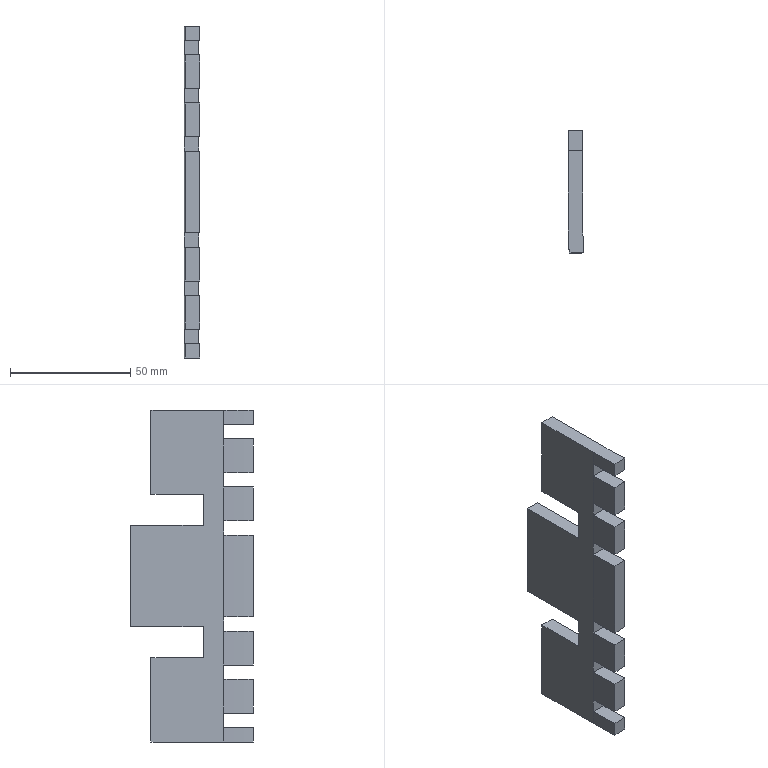Part | SolidWorks | features ICE 2, Extrusion 1 | 1 solid | 52 faces | box 6.316 x 51.1 x 138 mm | volume 31263 mm3 | plane 38 | cylinder 14 | commonest cylinder face diameters 461 x7 473 x7
STEP:
#1=CARTESIAN_POINT('',(-236.5,0.,69.));
#2=VERTEX_POINT('',#1);
#3=CARTESIAN_POINT('',(-236.5,0.,63.));
#4=VERTEX_POINT('',#3);
#5=CARTESIAN_POINT('',(-236.5,0.,69.));
#6=DIRECTION('',(0.,0.,-1.));
#7=VECTOR('',#6,1000.);
#8=LINE('',#5,#7);
#9=EDGE_CURVE('',#2,#4,#8,.T.);
#10=ORIENTED_EDGE('',*,*,#9,.T.);
#11=CARTESIAN_POINT('',(-236.176,-12.377,63.));
#12=VERTEX_POINT('',#11);
#13=CARTESIAN_POINT('',(0.,0.,63.));
#14=DIRECTION('',(0.,0.,1.));
#15=DIRECTION('',(1.,0.,0.));
#16=AXIS2_PLACEMENT_3D('',#13,#14,#15);
#17=CIRCLE('',#16,236.5);
#18=EDGE_CURVE('',#4,#12,#17,.T.);
#19=ORIENTED_EDGE('',*,*,#18,.T.);
#20=CARTESIAN_POINT('',(-236.176,-12.377,69.));
#21=VERTEX_POINT('',#20);
#22=CARTESIAN_POINT('',(-236.176,-12.377,69.));
#23=DIRECTION('',(0.,0.,-1.));
#24=VECTOR('',#23,1000.);
#25=LINE('',#22,#24);
#26=EDGE_CURVE('',#21,#12,#25,.T.);
#27=ORIENTED_EDGE('',*,*,#26,.F.);
#28=CARTESIAN_POINT('',(0.,0.,69.));
#29=DIRECTION('',(0.,0.,1.));
#30=DIRECTION('',(1.,0.,0.));
#31=AXIS2_PLACEMENT_3D('',#28,#29,#30);
#32=CIRCLE('',#31,236.5);
#33=EDGE_CURVE('',#2,#21,#32,.T.);
#34=ORIENTED_EDGE('',*,*,#33,.F.);
#35=EDGE_LOOP('',(#10,#19,#27,#34));
#36=FACE_OUTER_BOUND('',#35,.T.);
#37=CARTESIAN_POINT('',(0.,0.,69.));
#38=DIRECTION('',(0.,0.,-1.));
#39=DIRECTION('',(-1.,0.,0.));
#40=AXIS2_PLACEMENT_3D('',#37,#38,#39);
#41=CYLINDRICAL_SURFACE('',#40,236.5);
#42=ADVANCED_FACE('',(#36),#41,.T.);
#43=CARTESIAN_POINT('',(-236.176,-12.377,57.));
#44=VERTEX_POINT('',#43);
#45=CARTESIAN_POINT('',(-236.176,-12.377,43.));
#46=VERTEX_POINT('',#45);
#47=CARTESIAN_POINT('',(-236.176,-12.377,69.));
#48=DIRECTION('',(0.,0.,-1.));
#49=VECTOR('',#48,1000.);
#50=LINE('',#47,#49);
#51=EDGE_CURVE('',#44,#46,#50,.T.);
#52=ORIENTED_EDGE('',*,*,#51,.F.);
#53=CARTESIAN_POINT('',(-236.5,0.,57.));
#54=VERTEX_POINT('',#53);
#55=CARTESIAN_POINT('',(0.,0.,57.));
#56=DIRECTION('',(0.,0.,-1.));
#57=DIRECTION('',(-1.,0.,0.));
#58=AXIS2_PLACEMENT_3D('',#55,#56,#57);
#59=CIRCLE('',#58,236.5);
#60=EDGE_CURVE('',#44,#54,#59,.T.);
#61=ORIENTED_EDGE('',*,*,#60,.T.);
#62=CARTESIAN_POINT('',(-236.5,0.,43.));
#63=VERTEX_POINT('',#62);
#64=CARTESIAN_POINT('',(-236.5,0.,69.));
#65=DIRECTION('',(0.,0.,-1.));
#66=VECTOR('',#65,1000.);
#67=LINE('',#64,#66);
#68=EDGE_CURVE('',#54,#63,#67,.T.);
#69=ORIENTED_EDGE('',*,*,#68,.T.);
#70=CARTESIAN_POINT('',(0.,0.,43.));
#71=DIRECTION('',(0.,0.,1.));
#72=DIRECTION('',(1.,0.,0.));
#73=AXIS2_PLACEMENT_3D('',#70,#71,#72);
#74=CIRCLE('',#73,236.5);
#75=EDGE_CURVE('',#63,#46,#74,.T.);
#76=ORIENTED_EDGE('',*,*,#75,.T.);
#77=EDGE_LOOP('',(#52,#61,#69,#76));
#78=FACE_OUTER_BOUND('',#77,.T.);
#79=CARTESIAN_POINT('',(0.,0.,69.));
#80=DIRECTION('',(0.,0.,-1.));
#81=DIRECTION('',(-1.,0.,0.));
#82=AXIS2_PLACEMENT_3D('',#79,#80,#81);
#83=CYLINDRICAL_SURFACE('',#82,236.5);
#84=ADVANCED_FACE('',(#78),#83,.T.);
#85=CARTESIAN_POINT('',(-236.176,-12.377,37.));
#86=VERTEX_POINT('',#85);
#87=CARTESIAN_POINT('',(-236.176,-12.377,23.));
#88=VERTEX_POINT('',#87);
#89=CARTESIAN_POINT('',(-236.176,-12.377,69.));
#90=DIRECTION('',(0.,0.,-1.));
#91=VECTOR('',#90,1000.);
#92=LINE('',#89,#91);
#93=EDGE_CURVE('',#86,#88,#92,.T.);
#94=ORIENTED_EDGE('',*,*,#93,.F.);
#95=CARTESIAN_POINT('',(-236.5,0.,37.));
#96=VERTEX_POINT('',#95);
#97=CARTESIAN_POINT('',(0.,0.,37.));
#98=DIRECTION('',(0.,0.,-1.));
#99=DIRECTION('',(-1.,0.,0.));
#100=AXIS2_PLACEMENT_3D('',#97,#98,#99);
#101=CIRCLE('',#100,236.5);
#102=EDGE_CURVE('',#86,#96,#101,.T.);
#103=ORIENTED_EDGE('',*,*,#102,.T.);
#104=CARTESIAN_POINT('',(-236.5,0.,23.));
#105=VERTEX_POINT('',#104);
#106=CARTESIAN_POINT('',(-236.5,0.,69.));
#107=DIRECTION('',(0.,0.,-1.));
#108=VECTOR('',#107,1000.);
#109=LINE('',#106,#108);
#110=EDGE_CURVE('',#96,#105,#109,.T.);
#111=ORIENTED_EDGE('',*,*,#110,.T.);
#112=CARTESIAN_POINT('',(0.,0.,23.));
#113=DIRECTION('',(0.,0.,1.));
#114=DIRECTION('',(0.,-1.,0.));
#115=AXIS2_PLACEMENT_3D('',#112,#113,#114);
#116=CIRCLE('',#115,236.5);
#117=EDGE_CURVE('',#105,#88,#116,.T.);
#118=ORIENTED_EDGE('',*,*,#117,.T.);
#119=EDGE_LOOP('',(#94,#103,#111,#118));
#120=FACE_OUTER_BOUND('',#119,.T.);
#121=CARTESIAN_POINT('',(0.,0.,69.));
#122=DIRECTION('',(0.,0.,-1.));
#123=DIRECTION('',(-1.,0.,0.));
#124=AXIS2_PLACEMENT_3D('',#121,#122,#123);
#125=CYLINDRICAL_SURFACE('',#124,236.5);
#126=ADVANCED_FACE('',(#120),#125,.T.);
#127=CARTESIAN_POINT('',(-236.176,-12.377,17.));
#128=VERTEX_POINT('',#127);
#129=CARTESIAN_POINT('',(-236.176,-12.377,-17.));
#130=VERTEX_POINT('',#129);
#131=CARTESIAN_POINT('',(-236.176,-12.377,69.));
#132=DIRECTION('',(0.,0.,-1.));
#133=VECTOR('',#132,1000.);
#134=LINE('',#131,#133);
#135=EDGE_CURVE('',#128,#130,#134,.T.);
#136=ORIENTED_EDGE('',*,*,#135,.F.);
#137=CARTESIAN_POINT('',(-236.5,0.,17.));
#138=VERTEX_POINT('',#137);
#139=CARTESIAN_POINT('',(0.,0.,17.));
#140=DIRECTION('',(0.,0.,-1.));
#141=DIRECTION('',(0.,1.,0.));
#142=AXIS2_PLACEMENT_3D('',#139,#140,#141);
#143=CIRCLE('',#142,236.5);
#144=EDGE_CURVE('',#128,#138,#143,.T.);
#145=ORIENTED_EDGE('',*,*,#144,.T.);
#146=CARTESIAN_POINT('',(-236.5,0.,-17.));
#147=VERTEX_POINT('',#146);
#148=CARTESIAN_POINT('',(-236.5,0.,69.));
#149=DIRECTION('',(0.,0.,-1.));
#150=VECTOR('',#149,1000.);
#151=LINE('',#148,#150);
#152=EDGE_CURVE('',#138,#147,#151,.T.);
#153=ORIENTED_EDGE('',*,*,#152,.T.);
#154=CARTESIAN_POINT('',(0.,0.,-17.));
#155=DIRECTION('',(0.,0.,1.));
#156=DIRECTION('',(1.,0.,0.));
#157=AXIS2_PLACEMENT_3D('',#154,#155,#156);
#158=CIRCLE('',#157,236.5);
#159=EDGE_CURVE('',#147,#130,#158,.T.);
#160=ORIENTED_EDGE('',*,*,#159,.T.);
#161=EDGE_LOOP('',(#136,#145,#153,#160));
#162=FACE_OUTER_BOUND('',#161,.T.);
#163=CARTESIAN_POINT('',(0.,0.,69.));
#164=DIRECTION('',(0.,0.,-1.));
#165=DIRECTION('',(-1.,0.,0.));
#166=AXIS2_PLACEMENT_3D('',#163,#164,#165);
#167=CYLINDRICAL_SURFACE('',#166,236.5);
#168=ADVANCED_FACE('',(#162),#167,.T.);
#169=CARTESIAN_POINT('',(-236.176,-12.377,-23.));
#170=VERTEX_POINT('',#169);
#171=CARTESIAN_POINT('',(-236.176,-12.377,-37.));
#172=VERTEX_POINT('',#171);
#173=CARTESIAN_POINT('',(-236.176,-12.377,69.));
#174=DIRECTION('',(0.,0.,-1.));
#175=VECTOR('',#174,1000.);
#176=LINE('',#173,#175);
#177=EDGE_CURVE('',#170,#172,#176,.T.);
#178=ORIENTED_EDGE('',*,*,#177,.F.);
#179=CARTESIAN_POINT('',(-236.5,0.,-23.));
#180=VERTEX_POINT('',#179);
#181=CARTESIAN_POINT('',(0.,0.,-23.));
#182=DIRECTION('',(0.,0.,-1.));
#183=DIRECTION('',(0.,1.,0.));
#184=AXIS2_PLACEMENT_3D('',#181,#182,#183);
#185=CIRCLE('',#184,236.5);
#186=EDGE_CURVE('',#170,#180,#185,.T.);
#187=ORIENTED_EDGE('',*,*,#186,.T.);
#188=CARTESIAN_POINT('',(-236.5,0.,-37.));
#189=VERTEX_POINT('',#188);
#190=CARTESIAN_POINT('',(-236.5,0.,69.));
#191=DIRECTION('',(0.,0.,-1.));
#192=VECTOR('',#191,1000.);
#193=LINE('',#190,#192);
#194=EDGE_CURVE('',#180,#189,#193,.T.);
#195=ORIENTED_EDGE('',*,*,#194,.T.);
#196=CARTESIAN_POINT('',(0.,0.,-37.));
#197=DIRECTION('',(0.,0.,1.));
#198=DIRECTION('',(0.,-1.,0.));
#199=AXIS2_PLACEMENT_3D('',#196,#197,#198);
#200=CIRCLE('',#199,236.5);
#201=EDGE_CURVE('',#189,#172,#200,.T.);
#202=ORIENTED_EDGE('',*,*,#201,.T.);
#203=EDGE_LOOP('',(#178,#187,#195,#202));
#204=FACE_OUTER_BOUND('',#203,.T.);
#205=CARTESIAN_POINT('',(0.,0.,69.));
#206=DIRECTION('',(0.,0.,-1.));
#207=DIRECTION('',(-1.,0.,0.));
#208=AXIS2_PLACEMENT_3D('',#205,#206,#207);
#209=CYLINDRICAL_SURFACE('',#208,236.5);
#210=ADVANCED_FACE('',(#204),#209,.T.);
#211=CARTESIAN_POINT('',(-236.176,-12.377,-43.));
#212=VERTEX_POINT('',#211);
#213=CARTESIAN_POINT('',(-236.176,-12.377,-57.));
#214=VERTEX_POINT('',#213);
#215=CARTESIAN_POINT('',(-236.176,-12.377,69.));
#216=DIRECTION('',(0.,0.,-1.));
#217=VECTOR('',#216,1000.);
#218=LINE('',#215,#217);
#219=EDGE_CURVE('',#212,#214,#218,.T.);
#220=ORIENTED_EDGE('',*,*,#219,.F.);
#221=CARTESIAN_POINT('',(-236.5,0.,-43.));
#222=VERTEX_POINT('',#221);
#223=CARTESIAN_POINT('',(0.,0.,-43.));
#224=DIRECTION('',(0.,0.,-1.));
#225=DIRECTION('',(0.,1.,0.));
#226=AXIS2_PLACEMENT_3D('',#223,#224,#225);
#227=CIRCLE('',#226,236.5);
#228=EDGE_CURVE('',#212,#222,#227,.T.);
#229=ORIENTED_EDGE('',*,*,#228,.T.);
#230=CARTESIAN_POINT('',(-236.5,0.,-57.));
#231=VERTEX_POINT('',#230);
#232=CARTESIAN_POINT('',(-236.5,0.,69.));
#233=DIRECTION('',(0.,0.,-1.));
#234=VECTOR('',#233,1000.);
#235=LINE('',#232,#234);
#236=EDGE_CURVE('',#222,#231,#235,.T.);
#237=ORIENTED_EDGE('',*,*,#236,.T.);
#238=CARTESIAN_POINT('',(0.,0.,-57.));
#239=DIRECTION('',(0.,0.,1.));
#240=DIRECTION('',(0.,-1.,0.));
#241=AXIS2_PLACEMENT_3D('',#238,#239,#240);
#242=CIRCLE('',#241,236.5);
#243=EDGE_CURVE('',#231,#214,#242,.T.);
#244=ORIENTED_EDGE('',*,*,#243,.T.);
#245=EDGE_LOOP('',(#220,#229,#237,#244));
#246=FACE_OUTER_BOUND('',#245,.T.);
#247=CARTESIAN_POINT('',(0.,0.,69.));
#248=DIRECTION('',(0.,0.,-1.));
#249=DIRECTION('',(-1.,0.,0.));
#250=AXIS2_PLACEMENT_3D('',#247,#248,#249);
#251=CYLINDRICAL_SURFACE('',#250,236.5);
#252=ADVANCED_FACE('',(#246),#251,.T.);
#253=ORIENTED_EDGE('',*,*,#26,.T.);
#254=CARTESIAN_POINT('',(-230.184,-12.063,63.));
#255=VERTEX_POINT('',#254);
#256=CARTESIAN_POINT('',(-236.176,-12.377,63.));
#257=DIRECTION('',(0.9986,0.05234,0.));
#258=VECTOR('',#257,1000.);
#259=LINE('',#256,#258);
#260=EDGE_CURVE('',#12,#255,#259,.T.);
#261=ORIENTED_EDGE('',*,*,#260,.T.);
#262=CARTESIAN_POINT('',(-230.184,-12.063,69.));
#263=VERTEX_POINT('',#262);
#264=CARTESIAN_POINT('',(-230.184,-12.063,69.));
#265=DIRECTION('',(0.,0.,-1.));
#266=VECTOR('',#265,1000.);
#267=LINE('',#264,#266);
#268=EDGE_CURVE('',#263,#255,#267,.T.);
#269=ORIENTED_EDGE('',*,*,#268,.F.);
#270=CARTESIAN_POINT('',(-236.176,-12.377,69.));
#271=DIRECTION('',(0.9986,0.05234,0.));
#272=VECTOR('',#271,1000.);
#273=LINE('',#270,#272);
#274=EDGE_CURVE('',#21,#263,#273,.T.);
#275=ORIENTED_EDGE('',*,*,#274,.F.);
#276=EDGE_LOOP('',(#253,#261,#269,#275));
#277=FACE_OUTER_BOUND('',#276,.T.);
#278=CARTESIAN_POINT('',(-236.176,-12.377,69.));
#279=DIRECTION('',(-0.05234,0.9986,0.));
#280=DIRECTION('',(-0.9986,-0.05234,0.));
#281=AXIS2_PLACEMENT_3D('',#278,#279,#280);
#282=PLANE('',#281);
#283=ADVANCED_FACE('',(#277),#282,.F.);
#284=CARTESIAN_POINT('',(-230.184,-12.063,57.));
#285=VERTEX_POINT('',#284);
#286=CARTESIAN_POINT('',(-230.184,-12.063,43.));
#287=VERTEX_POINT('',#286);
#288=CARTESIAN_POINT('',(-230.184,-12.063,69.));
#289=DIRECTION('',(0.,0.,-1.));
#290=VECTOR('',#289,1000.);
#291=LINE('',#288,#290);
#292=EDGE_CURVE('',#285,#287,#291,.T.);
#293=ORIENTED_EDGE('',*,*,#292,.F.);
#294=CARTESIAN_POINT('',(-236.176,-12.377,57.));
#295=DIRECTION('',(-0.9986,-0.05234,0.));
#296=VECTOR('',#295,1000.);
#297=LINE('',#294,#296);
#298=EDGE_CURVE('',#285,#44,#297,.T.);
#299=ORIENTED_EDGE('',*,*,#298,.T.);
#300=ORIENTED_EDGE('',*,*,#51,.T.);
#301=CARTESIAN_POINT('',(-236.176,-12.377,43.));
#302=DIRECTION('',(0.9986,0.05234,0.));
#303=VECTOR('',#302,1000.);
#304=LINE('',#301,#303);
#305=EDGE_CURVE('',#46,#287,#304,.T.);
#306=ORIENTED_EDGE('',*,*,#305,.T.);
#307=EDGE_LOOP('',(#293,#299,#300,#306));
#308=FACE_OUTER_BOUND('',#307,.T.);
#309=CARTESIAN_POINT('',(-236.176,-12.377,69.));
#310=DIRECTION('',(-0.05234,0.9986,0.));
#311=DIRECTION('',(-0.9986,-0.05234,0.));
#312=AXIS2_PLACEMENT_3D('',#309,#310,#311);
#313=PLANE('',#312);
#314=ADVANCED_FACE('',(#308),#313,.F.);
#315=CARTESIAN_POINT('',(-230.184,-12.063,37.));
#316=VERTEX_POINT('',#315);
#317=CARTESIAN_POINT('',(-230.184,-12.063,23.));
#318=VERTEX_POINT('',#317);
#319=CARTESIAN_POINT('',(-230.184,-12.063,69.));
#320=DIRECTION('',(0.,0.,-1.));
#321=VECTOR('',#320,1000.);
#322=LINE('',#319,#321);
#323=EDGE_CURVE('',#316,#318,#322,.T.);
#324=ORIENTED_EDGE('',*,*,#323,.F.);
#325=CARTESIAN_POINT('',(-236.176,-12.377,37.));
#326=DIRECTION('',(-0.9986,-0.05234,0.));
#327=VECTOR('',#326,1000.);
#328=LINE('',#325,#327);
#329=EDGE_CURVE('',#316,#86,#328,.T.);
#330=ORIENTED_EDGE('',*,*,#329,.T.);
#331=ORIENTED_EDGE('',*,*,#93,.T.);
#332=CARTESIAN_POINT('',(-236.176,-12.377,23.));
#333=DIRECTION('',(0.9986,0.05234,0.));
#334=VECTOR('',#333,1000.);
#335=LINE('',#332,#334);
#336=EDGE_CURVE('',#88,#318,#335,.T.);
#337=ORIENTED_EDGE('',*,*,#336,.T.);
#338=EDGE_LOOP('',(#324,#330,#331,#337));
#339=FACE_OUTER_BOUND('',#338,.T.);
#340=CARTESIAN_POINT('',(-236.176,-12.377,69.));
#341=DIRECTION('',(-0.05234,0.9986,0.));
#342=DIRECTION('',(-0.9986,-0.05234,0.));
#343=AXIS2_PLACEMENT_3D('',#340,#341,#342);
#344=PLANE('',#343);
#345=ADVANCED_FACE('',(#339),#344,.F.);
#346=CARTESIAN_POINT('',(-230.184,-12.063,17.));
#347=VERTEX_POINT('',#346);
#348=CARTESIAN_POINT('',(-230.184,-12.063,-17.));
#349=VERTEX_POINT('',#348);
#350=CARTESIAN_POINT('',(-230.184,-12.063,69.));
#351=DIRECTION('',(0.,0.,-1.));
#352=VECTOR('',#351,1000.);
#353=LINE('',#350,#352);
#354=EDGE_CURVE('',#347,#349,#353,.T.);
#355=ORIENTED_EDGE('',*,*,#354,.F.);
#356=CARTESIAN_POINT('',(-236.176,-12.377,17.));
#357=DIRECTION('',(-0.9986,-0.05234,0.));
#358=VECTOR('',#357,1000.);
#359=LINE('',#356,#358);
#360=EDGE_CURVE('',#347,#128,#359,.T.);
#361=ORIENTED_EDGE('',*,*,#360,.T.);
#362=ORIENTED_EDGE('',*,*,#135,.T.);
#363=CARTESIAN_POINT('',(-236.176,-12.377,-17.));
#364=DIRECTION('',(0.9986,0.05234,0.));
#365=VECTOR('',#364,1000.);
#366=LINE('',#363,#365);
#367=EDGE_CURVE('',#130,#349,#366,.T.);
#368=ORIENTED_EDGE('',*,*,#367,.T.);
#369=EDGE_LOOP('',(#355,#361,#362,#368));
#370=FACE_OUTER_BOUND('',#369,.T.);
#371=CARTESIAN_POINT('',(-236.176,-12.377,69.));
#372=DIRECTION('',(-0.05234,0.9986,0.));
#373=DIRECTION('',(-0.9986,-0.05234,0.));
#374=AXIS2_PLACEMENT_3D('',#371,#372,#373);
#375=PLANE('',#374);
#376=ADVANCED_FACE('',(#370),#375,.F.);
#377=CARTESIAN_POINT('',(-230.184,-12.063,-23.));
#378=VERTEX_POINT('',#377);
#379=CARTESIAN_POINT('',(-230.184,-12.063,-37.));
#380=VERTEX_POINT('',#379);
#381=CARTESIAN_POINT('',(-230.184,-12.063,69.));
#382=DIRECTION('',(0.,0.,-1.));
#383=VECTOR('',#382,1000.);
#384=LINE('',#381,#383);
#385=EDGE_CURVE('',#378,#380,#384,.T.);
#386=ORIENTED_EDGE('',*,*,#385,.F.);
#387=CARTESIAN_POINT('',(-236.176,-12.377,-23.));
#388=DIRECTION('',(-0.9986,-0.05234,0.));
#389=VECTOR('',#388,1000.);
#390=LINE('',#387,#389);
#391=EDGE_CURVE('',#378,#170,#390,.T.);
#392=ORIENTED_EDGE('',*,*,#391,.T.);
#393=ORIENTED_EDGE('',*,*,#177,.T.);
#394=CARTESIAN_POINT('',(-236.176,-12.377,-37.));
#395=DIRECTION('',(0.9986,0.05234,0.));
#396=VECTOR('',#395,1000.);
#397=LINE('',#394,#396);
#398=EDGE_CURVE('',#172,#380,#397,.T.);
#399=ORIENTED_EDGE('',*,*,#398,.T.);
#400=EDGE_LOOP('',(#386,#392,#393,#399));
#401=FACE_OUTER_BOUND('',#400,.T.);
#402=CARTESIAN_POINT('',(-236.176,-12.377,69.));
#403=DIRECTION('',(-0.05234,0.9986,0.));
#404=DIRECTION('',(-0.9986,-0.05234,0.));
#405=AXIS2_PLACEMENT_3D('',#402,#403,#404);
#406=PLANE('',#405);
#407=ADVANCED_FACE('',(#401),#406,.F.);
#408=CARTESIAN_POINT('',(-230.184,-12.063,-43.));
#409=VERTEX_POINT('',#408);
#410=CARTESIAN_POINT('',(-230.184,-12.063,-57.));
#411=VERTEX_POINT('',#410);
#412=CARTESIAN_POINT('',(-230.184,-12.063,69.));
#413=DIRECTION('',(0.,0.,-1.));
#414=VECTOR('',#413,1000.);
#415=LINE('',#412,#414);
#416=EDGE_CURVE('',#409,#411,#415,.T.);
#417=ORIENTED_EDGE('',*,*,#416,.F.);
#418=CARTESIAN_POINT('',(-236.176,-12.377,-43.));
#419=DIRECTION('',(-0.9986,-0.05234,0.));
#420=VECTOR('',#419,1000.);
#421=LINE('',#418,#420);
#422=EDGE_CURVE('',#409,#212,#421,.T.);
#423=ORIENTED_EDGE('',*,*,#422,.T.);
#424=ORIENTED_EDGE('',*,*,#219,.T.);
#425=CARTESIAN_POINT('',(-236.176,-12.377,-57.));
#426=DIRECTION('',(0.9986,0.05234,0.));
#427=VECTOR('',#426,1000.);
#428=LINE('',#425,#427);
#429=EDGE_CURVE('',#214,#411,#428,.T.);
#430=ORIENTED_EDGE('',*,*,#429,.T.);
#431=EDGE_LOOP('',(#417,#423,#424,#430));
#432=FACE_OUTER_BOUND('',#431,.T.);
#433=CARTESIAN_POINT('',(-236.176,-12.377,69.));
#434=DIRECTION('',(-0.05234,0.9986,0.));
#435=DIRECTION('',(-0.9986,-0.05234,0.));
#436=AXIS2_PLACEMENT_3D('',#433,#434,#435);
#437=PLANE('',#436);
#438=ADVANCED_FACE('',(#432),#437,.F.);
#439=ORIENTED_EDGE('',*,*,#268,.T.);
#440=CARTESIAN_POINT('',(-230.5,0.,63.));
#441=VERTEX_POINT('',#440);
#442=CARTESIAN_POINT('',(0.,0.,63.));
#443=DIRECTION('',(0.,0.,-1.));
#444=DIRECTION('',(1.,0.,0.));
#445=AXIS2_PLACEMENT_3D('',#442,#443,#444);
#446=CIRCLE('',#445,230.5);
#447=EDGE_CURVE('',#255,#441,#446,.T.);
#448=ORIENTED_EDGE('',*,*,#447,.T.);
#449=CARTESIAN_POINT('',(-230.5,0.,69.));
#450=VERTEX_POINT('',#449);
#451=CARTESIAN_POINT('',(-230.5,0.,69.));
#452=DIRECTION('',(0.,0.,-1.));
#453=VECTOR('',#452,1000.);
#454=LINE('',#451,#453);
#455=EDGE_CURVE('',#450,#441,#454,.T.);
#456=ORIENTED_EDGE('',*,*,#455,.F.);
#457=CARTESIAN_POINT('',(0.,0.,69.));
#458=DIRECTION('',(0.,0.,-1.));
#459=DIRECTION('',(1.,0.,0.));
#460=AXIS2_PLACEMENT_3D('',#457,#458,#459);
#461=CIRCLE('',#460,230.5);
#462=EDGE_CURVE('',#263,#450,#461,.T.);
#463=ORIENTED_EDGE('',*,*,#462,.F.);
#464=EDGE_LOOP('',(#439,#448,#456,#463));
#465=FACE_OUTER_BOUND('',#464,.T.);
#466=CARTESIAN_POINT('',(0.,0.,69.));
#467=DIRECTION('',(0.,0.,-1.));
#468=DIRECTION('',(-1.,0.,0.));
#469=AXIS2_PLACEMENT_3D('',#466,#467,#468);
#470=CYLINDRICAL_SURFACE('',#469,230.5);
#471=ADVANCED_FACE('',(#465),#470,.F.);
#472=CARTESIAN_POINT('',(-230.5,0.,57.));
#473=VERTEX_POINT('',#472);
#474=CARTESIAN_POINT('',(-230.5,0.,43.));
#475=VERTEX_POINT('',#474);
#476=CARTESIAN_POINT('',(-230.5,0.,69.));
#477=DIRECTION('',(0.,0.,-1.));
#478=VECTOR('',#477,1000.);
#479=LINE('',#476,#478);
#480=EDGE_CURVE('',#473,#475,#479,.T.);
#481=ORIENTED_EDGE('',*,*,#480,.F.);
#482=CARTESIAN_POINT('',(0.,0.,57.));
#483=DIRECTION('',(0.,0.,1.));
#484=DIRECTION('',(-1.,0.,0.));
#485=AXIS2_PLACEMENT_3D('',#482,#483,#484);
#486=CIRCLE('',#485,230.5);
#487=EDGE_CURVE('',#473,#285,#486,.T.);
#488=ORIENTED_EDGE('',*,*,#487,.T.);
#489=ORIENTED_EDGE('',*,*,#292,.T.);
#490=CARTESIAN_POINT('',(0.,0.,43.));
#491=DIRECTION('',(0.,0.,-1.));
#492=DIRECTION('',(1.,0.,0.));
#493=AXIS2_PLACEMENT_3D('',#490,#491,#492);
#494=CIRCLE('',#493,230.5);
#495=EDGE_CURVE('',#287,#475,#494,.T.);
#496=ORIENTED_EDGE('',*,*,#495,.T.);
#497=EDGE_LOOP('',(#481,#488,#489,#496));
#498=FACE_OUTER_BOUND('',#497,.T.);
#499=CARTESIAN_POINT('',(0.,0.,69.));
#500=DIRECTION('',(0.,0.,-1.));
#501=DIRECTION('',(-1.,0.,0.));
#502=AXIS2_PLACEMENT_3D('',#499,#500,#501);
#503=CYLINDRICAL_SURFACE('',#502,230.5);
#504=ADVANCED_FACE('',(#498),#503,.F.);
#505=CARTESIAN_POINT('',(-230.5,0.,37.));
#506=VERTEX_POINT('',#505);
#507=CARTESIAN_POINT('',(-230.5,0.,23.));
#508=VERTEX_POINT('',#507);
#509=CARTESIAN_POINT('',(-230.5,0.,69.));
#510=DIRECTION('',(0.,0.,-1.));
#511=VECTOR('',#510,1000.);
#512=LINE('',#509,#511);
#513=EDGE_CURVE('',#506,#508,#512,.T.);
#514=ORIENTED_EDGE('',*,*,#513,.F.);
#515=CARTESIAN_POINT('',(0.,0.,37.));
#516=DIRECTION('',(0.,0.,1.));
#517=DIRECTION('',(-1.,0.,0.));
#518=AXIS2_PLACEMENT_3D('',#515,#516,#517);
#519=CIRCLE('',#518,230.5);
#520=EDGE_CURVE('',#506,#316,#519,.T.);
#521=ORIENTED_EDGE('',*,*,#520,.T.);
#522=ORIENTED_EDGE('',*,*,#323,.T.);
#523=CARTESIAN_POINT('',(0.,0.,23.));
#524=DIRECTION('',(0.,0.,-1.));
#525=DIRECTION('',(0.,-1.,0.));
#526=AXIS2_PLACEMENT_3D('',#523,#524,#525);
#527=CIRCLE('',#526,230.5);
#528=EDGE_CURVE('',#318,#508,#527,.T.);
#529=ORIENTED_EDGE('',*,*,#528,.T.);
#530=EDGE_LOOP('',(#514,#521,#522,#529));
#531=FACE_OUTER_BOUND('',#530,.T.);
#532=CARTESIAN_POINT('',(0.,0.,69.));
#533=DIRECTION('',(0.,0.,-1.));
#534=DIRECTION('',(-1.,0.,0.));
#535=AXIS2_PLACEMENT_3D('',#532,#533,#534);
#536=CYLINDRICAL_SURFACE('',#535,230.5);
#537=ADVANCED_FACE('',(#531),#536,.F.);
#538=CARTESIAN_POINT('',(-230.5,0.,17.));
#539=VERTEX_POINT('',#538);
#540=CARTESIAN_POINT('',(-230.5,0.,-17.));
#541=VERTEX_POINT('',#540);
#542=CARTESIAN_POINT('',(-230.5,0.,69.));
#543=DIRECTION('',(0.,0.,-1.));
#544=VECTOR('',#543,1000.);
#545=LINE('',#542,#544);
#546=EDGE_CURVE('',#539,#541,#545,.T.);
#547=ORIENTED_EDGE('',*,*,#546,.F.);
#548=CARTESIAN_POINT('',(0.,0.,17.));
#549=DIRECTION('',(0.,0.,1.));
#550=DIRECTION('',(0.,1.,0.));
#551=AXIS2_PLACEMENT_3D('',#548,#549,#550);
#552=CIRCLE('',#551,230.5);
#553=EDGE_CURVE('',#539,#347,#552,.T.);
#554=ORIENTED_EDGE('',*,*,#553,.T.);
#555=ORIENTED_EDGE('',*,*,#354,.T.);
#556=CARTESIAN_POINT('',(0.,0.,-17.));
#557=DIRECTION('',(0.,0.,-1.));
#558=DIRECTION('',(1.,0.,0.));
#559=AXIS2_PLACEMENT_3D('',#556,#557,#558);
#560=CIRCLE('',#559,230.5);
#561=EDGE_CURVE('',#349,#541,#560,.T.);
#562=ORIENTED_EDGE('',*,*,#561,.T.);
#563=EDGE_LOOP('',(#547,#554,#555,#562));
#564=FACE_OUTER_BOUND('',#563,.T.);
#565=CARTESIAN_POINT('',(0.,0.,69.));
#566=DIRECTION('',(0.,0.,-1.));
#567=DIRECTION('',(-1.,0.,0.));
#568=AXIS2_PLACEMENT_3D('',#565,#566,#567);
#569=CYLINDRICAL_SURFACE('',#568,230.5);
#570=ADVANCED_FACE('',(#564),#569,.F.);
#571=CARTESIAN_POINT('',(-230.5,0.,-23.));
#572=VERTEX_POINT('',#571);
#573=CARTESIAN_POINT('',(-230.5,0.,-37.));
#574=VERTEX_POINT('',#573);
#575=CARTESIAN_POINT('',(-230.5,0.,69.));
#576=DIRECTION('',(0.,0.,-1.));
#577=VECTOR('',#576,1000.);
#578=LINE('',#575,#577);
#579=EDGE_CURVE('',#572,#574,#578,.T.);
#580=ORIENTED_EDGE('',*,*,#579,.F.);
#581=CARTESIAN_POINT('',(0.,0.,-23.));
#582=DIRECTION('',(0.,0.,1.));
#583=DIRECTION('',(0.,1.,0.));
#584=AXIS2_PLACEMENT_3D('',#581,#582,#583);
#585=CIRCLE('',#584,230.5);
#586=EDGE_CURVE('',#572,#378,#585,.T.);
#587=ORIENTED_EDGE('',*,*,#586,.T.);
#588=ORIENTED_EDGE('',*,*,#385,.T.);
#589=CARTESIAN_POINT('',(0.,0.,-37.));
#590=DIRECTION('',(0.,0.,-1.));
#591=DIRECTION('',(0.,-1.,0.));
#592=AXIS2_PLACEMENT_3D('',#589,#590,#591);
#593=CIRCLE('',#592,230.5);
#594=EDGE_CURVE('',#380,#574,#593,.T.);
#595=ORIENTED_EDGE('',*,*,#594,.T.);
#596=EDGE_LOOP('',(#580,#587,#588,#595));
#597=FACE_OUTER_BOUND('',#596,.T.);
#598=CARTESIAN_POINT('',(0.,0.,69.));
#599=DIRECTION('',(0.,0.,-1.));
#600=DIRECTION('',(-1.,0.,0.));
#601=AXIS2_PLACEMENT_3D('',#598,#599,#600);
#602=CYLINDRICAL_SURFACE('',#601,230.5);
#603=ADVANCED_FACE('',(#597),#602,.F.);
#604=CARTESIAN_POINT('',(-230.5,0.,-43.));
#605=VERTEX_POINT('',#604);
#606=CARTESIAN_POINT('',(-230.5,0.,-57.));
#607=VERTEX_POINT('',#606);
#608=CARTESIAN_POINT('',(-230.5,0.,69.));
#609=DIRECTION('',(0.,0.,-1.));
#610=VECTOR('',#609,1000.);
#611=LINE('',#608,#610);
#612=EDGE_CURVE('',#605,#607,#611,.T.);
#613=ORIENTED_EDGE('',*,*,#612,.F.);
#614=CARTESIAN_POINT('',(0.,0.,-43.));
#615=DIRECTION('',(0.,0.,1.));
#616=DIRECTION('',(0.,1.,0.));
#617=AXIS2_PLACEMENT_3D('',#614,#615,#616);
#618=CIRCLE('',#617,230.5);
#619=EDGE_CURVE('',#605,#409,#618,.T.);
#620=ORIENTED_EDGE('',*,*,#619,.T.);
#621=ORIENTED_EDGE('',*,*,#416,.T.);
#622=CARTESIAN_POINT('',(0.,0.,-57.));
#623=DIRECTION('',(0.,0.,-1.));
#624=DIRECTION('',(0.,-1.,0.));
#625=AXIS2_PLACEMENT_3D('',#622,#623,#624);
#626=CIRCLE('',#625,230.5);
#627=EDGE_CURVE('',#411,#607,#626,.T.);
#628=ORIENTED_EDGE('',*,*,#627,.T.);
#629=EDGE_LOOP('',(#613,#620,#621,#628));
#630=FACE_OUTER_BOUND('',#629,.T.);
#631=CARTESIAN_POINT('',(0.,0.,69.));
#632=DIRECTION('',(0.,0.,-1.));
#633=DIRECTION('',(-1.,0.,0.));
#634=AXIS2_PLACEMENT_3D('',#631,#632,#633);
#635=CYLINDRICAL_SURFACE('',#634,230.5);
#636=ADVANCED_FACE('',(#630),#635,.F.);
#637=CARTESIAN_POINT('',(-236.176,-12.377,-63.));
#638=VERTEX_POINT('',#637);
#639=CARTESIAN_POINT('',(-236.176,-12.377,-69.));
#640=VERTEX_POINT('',#639);
#641=CARTESIAN_POINT('',(-236.176,-12.377,69.));
#642=DIRECTION('',(0.,0.,-1.));
#643=VECTOR('',#642,1000.);
#644=LINE('',#641,#643);
#645=EDGE_CURVE('',#638,#640,#644,.T.);
#646=ORIENTED_EDGE('',*,*,#645,.F.);
#647=CARTESIAN_POINT('',(-236.5,0.,-63.));
#648=VERTEX_POINT('',#647);
#649=CARTESIAN_POINT('',(0.,0.,-63.));
#650=DIRECTION('',(0.,0.,-1.));
#651=DIRECTION('',(-1.,0.,0.));
#652=AXIS2_PLACEMENT_3D('',#649,#650,#651);
#653=CIRCLE('',#652,236.5);
#654=EDGE_CURVE('',#638,#648,#653,.T.);
#655=ORIENTED_EDGE('',*,*,#654,.T.);
#656=CARTESIAN_POINT('',(-236.5,0.,-69.));
#657=VERTEX_POINT('',#656);
#658=CARTESIAN_POINT('',(-236.5,0.,69.));
#659=DIRECTION('',(0.,0.,-1.));
#660=VECTOR('',#659,1000.);
#661=LINE('',#658,#660);
#662=EDGE_CURVE('',#648,#657,#661,.T.);
#663=ORIENTED_EDGE('',*,*,#662,.T.);
#664=CARTESIAN_POINT('',(0.,0.,-69.));
#665=DIRECTION('',(0.,0.,1.));
#666=DIRECTION('',(1.,0.,0.));
#667=AXIS2_PLACEMENT_3D('',#664,#665,#666);
#668=CIRCLE('',#667,236.5);
#669=EDGE_CURVE('',#657,#640,#668,.T.);
#670=ORIENTED_EDGE('',*,*,#669,.T.);
#671=EDGE_LOOP('',(#646,#655,#663,#670));
#672=FACE_OUTER_BOUND('',#671,.T.);
#673=CARTESIAN_POINT('',(0.,0.,69.));
#674=DIRECTION('',(0.,0.,-1.));
#675=DIRECTION('',(-1.,0.,0.));
#676=AXIS2_PLACEMENT_3D('',#673,#674,#675);
#677=CYLINDRICAL_SURFACE('',#676,236.5);
#678=ADVANCED_FACE('',(#672),#677,.T.);
#679=CARTESIAN_POINT('',(-230.184,-12.063,-63.));
#680=VERTEX_POINT('',#679);
#681=CARTESIAN_POINT('',(-230.184,-12.063,-69.));
#682=VERTEX_POINT('',#681);
#683=CARTESIAN_POINT('',(-230.184,-12.063,69.));
#684=DIRECTION('',(0.,0.,-1.));
#685=VECTOR('',#684,1000.);
#686=LINE('',#683,#685);
#687=EDGE_CURVE('',#680,#682,#686,.T.);
#688=ORIENTED_EDGE('',*,*,#687,.F.);
#689=CARTESIAN_POINT('',(-236.176,-12.377,-63.));
#690=DIRECTION('',(-0.9986,-0.05234,0.));
#691=VECTOR('',#690,1000.);
#692=LINE('',#689,#691);
#693=EDGE_CURVE('',#680,#638,#692,.T.);
#694=ORIENTED_EDGE('',*,*,#693,.T.);
#695=ORIENTED_EDGE('',*,*,#645,.T.);
#696=CARTESIAN_POINT('',(-236.176,-12.377,-69.));
#697=DIRECTION('',(0.9986,0.05234,0.));
#698=VECTOR('',#697,1000.);
#699=LINE('',#696,#698);
#700=EDGE_CURVE('',#640,#682,#699,.T.);
#701=ORIENTED_EDGE('',*,*,#700,.T.);
#702=EDGE_LOOP('',(#688,#694,#695,#701));
#703=FACE_OUTER_BOUND('',#702,.T.);
#704=CARTESIAN_POINT('',(-236.176,-12.377,69.));
#705=DIRECTION('',(-0.05234,0.9986,0.));
#706=DIRECTION('',(-0.9986,-0.05234,0.));
#707=AXIS2_PLACEMENT_3D('',#704,#705,#706);
#708=PLANE('',#707);
#709=ADVANCED_FACE('',(#703),#708,.F.);
#710=CARTESIAN_POINT('',(-230.5,0.,-63.));
#711=VERTEX_POINT('',#710);
#712=CARTESIAN_POINT('',(-230.5,0.,-69.));
#713=VERTEX_POINT('',#712);
#714=CARTESIAN_POINT('',(-230.5,0.,69.));
#715=DIRECTION('',(0.,0.,-1.));
#716=VECTOR('',#715,1000.);
#717=LINE('',#714,#716);
#718=EDGE_CURVE('',#711,#713,#717,.T.);
#719=ORIENTED_EDGE('',*,*,#718,.F.);
#720=CARTESIAN_POINT('',(0.,0.,-63.));
#721=DIRECTION('',(0.,0.,1.));
#722=DIRECTION('',(-1.,0.,0.));
#723=AXIS2_PLACEMENT_3D('',#720,#721,#722);
#724=CIRCLE('',#723,230.5);
#725=EDGE_CURVE('',#711,#680,#724,.T.);
#726=ORIENTED_EDGE('',*,*,#725,.T.);
#727=ORIENTED_EDGE('',*,*,#687,.T.);
#728=CARTESIAN_POINT('',(0.,0.,-69.));
#729=DIRECTION('',(0.,0.,-1.));
#730=DIRECTION('',(1.,0.,0.));
#731=AXIS2_PLACEMENT_3D('',#728,#729,#730);
#732=CIRCLE('',#731,230.5);
#733=EDGE_CURVE('',#682,#713,#732,.T.);
#734=ORIENTED_EDGE('',*,*,#733,.T.);
#735=EDGE_LOOP('',(#719,#726,#727,#734));
#736=FACE_OUTER_BOUND('',#735,.T.);
#737=CARTESIAN_POINT('',(0.,0.,69.));
#738=DIRECTION('',(0.,0.,-1.));
#739=DIRECTION('',(-1.,0.,0.));
#740=AXIS2_PLACEMENT_3D('',#737,#738,#739);
#741=CYLINDRICAL_SURFACE('',#740,230.5);
#742=ADVANCED_FACE('',(#736),#741,.F.);
#743=CARTESIAN_POINT('',(-230.5,38.723,21.));
#744=VERTEX_POINT('',#743);
#745=CARTESIAN_POINT('',(-230.5,38.723,-21.));
#746=VERTEX_POINT('',#745);
#747=CARTESIAN_POINT('',(-230.5,38.723,69.));
#748=DIRECTION('',(0.,0.,-1.));
#749=VECTOR('',#748,1000.);
#750=LINE('',#747,#749);
#751=EDGE_CURVE('',#744,#746,#750,.T.);
#752=ORIENTED_EDGE('',*,*,#751,.F.);
#753=CARTESIAN_POINT('',(-230.5,8.523,21.));
#754=VERTEX_POINT('',#753);
#755=CARTESIAN_POINT('',(-230.5,8.523,21.));
#756=DIRECTION('',(0.,1.,0.));
#757=VECTOR('',#756,1000.);
#758=LINE('',#755,#757);
#759=EDGE_CURVE('',#754,#744,#758,.T.);
#760=ORIENTED_EDGE('',*,*,#759,.F.);
#761=CARTESIAN_POINT('',(-230.5,8.523,34.));
#762=VERTEX_POINT('',#761);
#763=CARTESIAN_POINT('',(-230.5,8.523,34.));
#764=DIRECTION('',(0.,0.,-1.));
#765=VECTOR('',#764,1000.);
#766=LINE('',#763,#765);
#767=EDGE_CURVE('',#762,#754,#766,.T.);
#768=ORIENTED_EDGE('',*,*,#767,.F.);
#769=CARTESIAN_POINT('',(-230.5,30.223,34.));
#770=VERTEX_POINT('',#769);
#771=CARTESIAN_POINT('',(-230.5,30.223,34.));
#772=DIRECTION('',(0.,-1.,0.));
#773=VECTOR('',#772,1000.);
#774=LINE('',#771,#773);
#775=EDGE_CURVE('',#770,#762,#774,.T.);
#776=ORIENTED_EDGE('',*,*,#775,.F.);
#777=CARTESIAN_POINT('',(-230.5,30.223,69.));
#778=VERTEX_POINT('',#777);
#779=CARTESIAN_POINT('',(-230.5,30.223,69.));
#780=DIRECTION('',(0.,0.,-1.));
#781=VECTOR('',#780,1000.);
#782=LINE('',#779,#781);
#783=EDGE_CURVE('',#778,#770,#782,.T.);
#784=ORIENTED_EDGE('',*,*,#783,.F.);
#785=CARTESIAN_POINT('',(-230.5,0.,69.));
#786=DIRECTION('',(0.,1.,0.));
#787=VECTOR('',#786,1000.);
#788=LINE('',#785,#787);
#789=EDGE_CURVE('',#450,#778,#788,.T.);
#790=ORIENTED_EDGE('',*,*,#789,.F.);
#791=ORIENTED_EDGE('',*,*,#455,.T.);
#792=CARTESIAN_POINT('',(-230.5,0.,69.));
#793=DIRECTION('',(0.,0.,-1.));
#794=VECTOR('',#793,1000.);
#795=LINE('',#792,#794);
#796=EDGE_CURVE('',#441,#473,#795,.T.);
#797=ORIENTED_EDGE('',*,*,#796,.T.);
#798=ORIENTED_EDGE('',*,*,#480,.T.);
#799=CARTESIAN_POINT('',(-230.5,0.,69.));
#800=DIRECTION('',(0.,0.,-1.));
#801=VECTOR('',#800,1000.);
#802=LINE('',#799,#801);
#803=EDGE_CURVE('',#475,#506,#802,.T.);
#804=ORIENTED_EDGE('',*,*,#803,.T.);
#805=ORIENTED_EDGE('',*,*,#513,.T.);
#806=CARTESIAN_POINT('',(-230.5,0.,69.));
#807=DIRECTION('',(0.,0.,-1.));
#808=VECTOR('',#807,1000.);
#809=LINE('',#806,#808);
#810=EDGE_CURVE('',#508,#539,#809,.T.);
#811=ORIENTED_EDGE('',*,*,#810,.T.);
#812=ORIENTED_EDGE('',*,*,#546,.T.);
#813=CARTESIAN_POINT('',(-230.5,0.,69.));
#814=DIRECTION('',(0.,0.,-1.));
#815=VECTOR('',#814,1000.);
#816=LINE('',#813,#815);
#817=EDGE_CURVE('',#541,#572,#816,.T.);
#818=ORIENTED_EDGE('',*,*,#817,.T.);
#819=ORIENTED_EDGE('',*,*,#579,.T.);
#820=CARTESIAN_POINT('',(-230.5,0.,69.));
#821=DIRECTION('',(0.,0.,-1.));
#822=VECTOR('',#821,1000.);
#823=LINE('',#820,#822);
#824=EDGE_CURVE('',#574,#605,#823,.T.);
#825=ORIENTED_EDGE('',*,*,#824,.T.);
#826=ORIENTED_EDGE('',*,*,#612,.T.);
#827=CARTESIAN_POINT('',(-230.5,0.,69.));
#828=DIRECTION('',(0.,0.,-1.));
#829=VECTOR('',#828,1000.);
#830=LINE('',#827,#829);
#831=EDGE_CURVE('',#607,#711,#830,.T.);
#832=ORIENTED_EDGE('',*,*,#831,.T.);
#833=ORIENTED_EDGE('',*,*,#718,.T.);
#834=CARTESIAN_POINT('',(-230.5,30.223,-69.));
#835=VERTEX_POINT('',#834);
#836=CARTESIAN_POINT('',(-230.5,0.,-69.));
#837=DIRECTION('',(0.,1.,0.));
#838=VECTOR('',#837,1000.);
#839=LINE('',#836,#838);
#840=EDGE_CURVE('',#713,#835,#839,.T.);
#841=ORIENTED_EDGE('',*,*,#840,.T.);
#842=CARTESIAN_POINT('',(-230.5,30.223,-34.));
#843=VERTEX_POINT('',#842);
#844=CARTESIAN_POINT('',(-230.5,30.223,-69.));
#845=DIRECTION('',(0.,0.,-1.));
#846=VECTOR('',#845,1000.);
#847=LINE('',#844,#846);
#848=EDGE_CURVE('',#843,#835,#847,.T.);
#849=ORIENTED_EDGE('',*,*,#848,.F.);
#850=CARTESIAN_POINT('',(-230.5,8.523,-34.));
#851=VERTEX_POINT('',#850);
#852=CARTESIAN_POINT('',(-230.5,30.223,-34.));
#853=DIRECTION('',(0.,1.,0.));
#854=VECTOR('',#853,1000.);
#855=LINE('',#852,#854);
#856=EDGE_CURVE('',#851,#843,#855,.T.);
#857=ORIENTED_EDGE('',*,*,#856,.F.);
#858=CARTESIAN_POINT('',(-230.5,8.523,-21.));
#859=VERTEX_POINT('',#858);
#860=CARTESIAN_POINT('',(-230.5,8.523,-34.));
#861=DIRECTION('',(0.,0.,-1.));
#862=VECTOR('',#861,1000.);
#863=LINE('',#860,#862);
#864=EDGE_CURVE('',#859,#851,#863,.T.);
#865=ORIENTED_EDGE('',*,*,#864,.F.);
#866=CARTESIAN_POINT('',(-230.5,8.523,-21.));
#867=DIRECTION('',(0.,-1.,0.));
#868=VECTOR('',#867,1000.);
#869=LINE('',#866,#868);
#870=EDGE_CURVE('',#746,#859,#869,.T.);
#871=ORIENTED_EDGE('',*,*,#870,.F.);
#872=EDGE_LOOP('',(#752,#760,#768,#776,#784,#790,#791,#797,#798,#804,#805,#811,#812,#818,#819,#825,#826,#832,#833,#841,#849,#857,#865,#871));
#873=FACE_OUTER_BOUND('',#872,.T.);
#874=CARTESIAN_POINT('',(-230.5,0.,69.));
#875=DIRECTION('',(-1.,0.,0.));
#876=DIRECTION('',(0.,0.,1.));
#877=AXIS2_PLACEMENT_3D('',#874,#875,#876);
#878=PLANE('',#877);
#879=ADVANCED_FACE('',(#873),#878,.F.);
#880=CARTESIAN_POINT('',(-236.5,38.723,21.));
#881=VERTEX_POINT('',#880);
#882=CARTESIAN_POINT('',(-236.5,38.723,-21.));
#883=VERTEX_POINT('',#882);
#884=CARTESIAN_POINT('',(-236.5,38.723,69.));
#885=DIRECTION('',(0.,0.,-1.));
#886=VECTOR('',#885,1000.);
#887=LINE('',#884,#886);
#888=EDGE_CURVE('',#881,#883,#887,.T.);
#889=ORIENTED_EDGE('',*,*,#888,.F.);
#890=CARTESIAN_POINT('',(-236.5,38.723,21.));
#891=DIRECTION('',(1.,0.,0.));
#892=VECTOR('',#891,1000.);
#893=LINE('',#890,#892);
#894=EDGE_CURVE('',#881,#744,#893,.T.);
#895=ORIENTED_EDGE('',*,*,#894,.T.);
#896=ORIENTED_EDGE('',*,*,#751,.T.);
#897=CARTESIAN_POINT('',(-236.5,38.723,-21.));
#898=DIRECTION('',(1.,0.,0.));
#899=VECTOR('',#898,1000.);
#900=LINE('',#897,#899);
#901=EDGE_CURVE('',#883,#746,#900,.T.);
#902=ORIENTED_EDGE('',*,*,#901,.F.);
#903=EDGE_LOOP('',(#889,#895,#896,#902));
#904=FACE_OUTER_BOUND('',#903,.T.);
#905=CARTESIAN_POINT('',(-236.5,38.723,69.));
#906=DIRECTION('',(0.,-1.,0.));
#907=DIRECTION('',(1.,0.,0.));
#908=AXIS2_PLACEMENT_3D('',#905,#906,#907);
#909=PLANE('',#908);
#910=ADVANCED_FACE('',(#904),#909,.F.);
#911=CARTESIAN_POINT('',(-236.5,8.523,34.));
#912=VERTEX_POINT('',#911);
#913=CARTESIAN_POINT('',(-236.5,8.523,21.));
#914=VERTEX_POINT('',#913);
#915=CARTESIAN_POINT('',(-236.5,8.523,34.));
#916=DIRECTION('',(0.,0.,-1.));
#917=VECTOR('',#916,1000.);
#918=LINE('',#915,#917);
#919=EDGE_CURVE('',#912,#914,#918,.T.);
#920=ORIENTED_EDGE('',*,*,#919,.T.);
#921=CARTESIAN_POINT('',(-236.5,8.523,21.));
#922=DIRECTION('',(0.,1.,0.));
#923=VECTOR('',#922,1000.);
#924=LINE('',#921,#923);
#925=EDGE_CURVE('',#914,#881,#924,.T.);
#926=ORIENTED_EDGE('',*,*,#925,.T.);
#927=ORIENTED_EDGE('',*,*,#888,.T.);
#928=CARTESIAN_POINT('',(-236.5,8.523,-21.));
#929=VERTEX_POINT('',#928);
#930=CARTESIAN_POINT('',(-236.5,8.523,-21.));
#931=DIRECTION('',(0.,-1.,0.));
#932=VECTOR('',#931,1000.);
#933=LINE('',#930,#932);
#934=EDGE_CURVE('',#883,#929,#933,.T.);
#935=ORIENTED_EDGE('',*,*,#934,.T.);
#936=CARTESIAN_POINT('',(-236.5,8.523,-34.));
#937=VERTEX_POINT('',#936);
#938=CARTESIAN_POINT('',(-236.5,8.523,-34.));
#939=DIRECTION('',(0.,0.,-1.));
#940=VECTOR('',#939,1000.);
#941=LINE('',#938,#940);
#942=EDGE_CURVE('',#929,#937,#941,.T.);
#943=ORIENTED_EDGE('',*,*,#942,.T.);
#944=CARTESIAN_POINT('',(-236.5,30.223,-34.));
#945=VERTEX_POINT('',#944);
#946=CARTESIAN_POINT('',(-236.5,30.223,-34.));
#947=DIRECTION('',(0.,1.,0.));
#948=VECTOR('',#947,1000.);
#949=LINE('',#946,#948);
#950=EDGE_CURVE('',#937,#945,#949,.T.);
#951=ORIENTED_EDGE('',*,*,#950,.T.);
#952=CARTESIAN_POINT('',(-236.5,30.223,-69.));
#953=VERTEX_POINT('',#952);
#954=CARTESIAN_POINT('',(-236.5,30.223,-69.));
#955=DIRECTION('',(0.,0.,-1.));
#956=VECTOR('',#955,1000.);
#957=LINE('',#954,#956);
#958=EDGE_CURVE('',#945,#953,#957,.T.);
#959=ORIENTED_EDGE('',*,*,#958,.T.);
#960=CARTESIAN_POINT('',(-236.5,0.,-69.));
#961=DIRECTION('',(0.,-1.,0.));
#962=VECTOR('',#961,1000.);
#963=LINE('',#960,#962);
#964=EDGE_CURVE('',#953,#657,#963,.T.);
#965=ORIENTED_EDGE('',*,*,#964,.T.);
#966=ORIENTED_EDGE('',*,*,#662,.F.);
#967=CARTESIAN_POINT('',(-236.5,0.,-63.));
#968=DIRECTION('',(0.,0.,1.));
#969=VECTOR('',#968,1000.);
#970=LINE('',#967,#969);
#971=EDGE_CURVE('',#648,#231,#970,.T.);
#972=ORIENTED_EDGE('',*,*,#971,.T.);
#973=ORIENTED_EDGE('',*,*,#236,.F.);
#974=CARTESIAN_POINT('',(-236.5,0.,-43.));
#975=DIRECTION('',(0.,0.,1.));
#976=VECTOR('',#975,1000.);
#977=LINE('',#974,#976);
#978=EDGE_CURVE('',#222,#189,#977,.T.);
#979=ORIENTED_EDGE('',*,*,#978,.T.);
#980=ORIENTED_EDGE('',*,*,#194,.F.);
#981=CARTESIAN_POINT('',(-236.5,0.,-23.));
#982=DIRECTION('',(0.,0.,1.));
#983=VECTOR('',#982,1000.);
#984=LINE('',#981,#983);
#985=EDGE_CURVE('',#180,#147,#984,.T.);
#986=ORIENTED_EDGE('',*,*,#985,.T.);
#987=ORIENTED_EDGE('',*,*,#152,.F.);
#988=CARTESIAN_POINT('',(-236.5,0.,23.));
#989=DIRECTION('',(0.,0.,1.));
#990=VECTOR('',#989,1000.);
#991=LINE('',#988,#990);
#992=EDGE_CURVE('',#138,#105,#991,.T.);
#993=ORIENTED_EDGE('',*,*,#992,.T.);
#994=ORIENTED_EDGE('',*,*,#110,.F.);
#995=CARTESIAN_POINT('',(-236.5,0.,43.));
#996=DIRECTION('',(0.,0.,1.));
#997=VECTOR('',#996,1000.);
#998=LINE('',#995,#997);
#999=EDGE_CURVE('',#96,#63,#998,.T.);
#1000=ORIENTED_EDGE('',*,*,#999,.T.);
#1001=ORIENTED_EDGE('',*,*,#68,.F.);
#1002=CARTESIAN_POINT('',(-236.5,0.,63.));
#1003=DIRECTION('',(0.,0.,1.));
#1004=VECTOR('',#1003,1000.);
#1005=LINE('',#1002,#1004);
#1006=EDGE_CURVE('',#54,#4,#1005,.T.);
#1007=ORIENTED_EDGE('',*,*,#1006,.T.);
#1008=ORIENTED_EDGE('',*,*,#9,.F.);
#1009=CARTESIAN_POINT('',(-236.5,30.223,69.));
#1010=VERTEX_POINT('',#1009);
#1011=CARTESIAN_POINT('',(-236.5,0.,69.));
#1012=DIRECTION('',(0.,-1.,0.));
#1013=VECTOR('',#1012,1000.);
#1014=LINE('',#1011,#1013);
#1015=EDGE_CURVE('',#1010,#2,#1014,.T.);
#1016=ORIENTED_EDGE('',*,*,#1015,.F.);
#1017=CARTESIAN_POINT('',(-236.5,30.223,34.));
#1018=VERTEX_POINT('',#1017);
#1019=CARTESIAN_POINT('',(-236.5,30.223,69.));
#1020=DIRECTION('',(0.,0.,-1.));
#1021=VECTOR('',#1020,1000.);
#1022=LINE('',#1019,#1021);
#1023=EDGE_CURVE('',#1010,#1018,#1022,.T.);
#1024=ORIENTED_EDGE('',*,*,#1023,.T.);
#1025=CARTESIAN_POINT('',(-236.5,30.223,34.));
#1026=DIRECTION('',(0.,-1.,0.));
#1027=VECTOR('',#1026,1000.);
#1028=LINE('',#1025,#1027);
#1029=EDGE_CURVE('',#1018,#912,#1028,.T.);
#1030=ORIENTED_EDGE('',*,*,#1029,.T.);
#1031=EDGE_LOOP('',(#920,#926,#927,#935,#943,#951,#959,#965,#966,#972,#973,#979,#980,#986,#987,#993,#994,#1000,#1001,#1007,#1008,#1016,#1024,#1030));
#1032=FACE_OUTER_BOUND('',#1031,.T.);
#1033=CARTESIAN_POINT('',(-236.5,0.,69.));
#1034=DIRECTION('',(1.,0.,0.));
#1035=DIRECTION('',(0.,1.,0.));
#1036=AXIS2_PLACEMENT_3D('',#1033,#1034,#1035);
#1037=PLANE('',#1036);
#1038=ADVANCED_FACE('',(#1032),#1037,.F.);
#1039=CARTESIAN_POINT('',(-236.5,30.223,69.));
#1040=DIRECTION('',(1.,0.,0.));
#1041=VECTOR('',#1040,1000.);
#1042=LINE('',#1039,#1041);
#1043=EDGE_CURVE('',#1010,#778,#1042,.T.);
#1044=ORIENTED_EDGE('',*,*,#1043,.F.);
#1045=ORIENTED_EDGE('',*,*,#1015,.T.);
#1046=ORIENTED_EDGE('',*,*,#33,.T.);
#1047=ORIENTED_EDGE('',*,*,#274,.T.);
#1048=ORIENTED_EDGE('',*,*,#462,.T.);
#1049=ORIENTED_EDGE('',*,*,#789,.T.);
#1050=EDGE_LOOP('',(#1044,#1045,#1046,#1047,#1048,#1049));
#1051=FACE_OUTER_BOUND('',#1050,.T.);
#1052=CARTESIAN_POINT('',(0.,0.,69.));
#1053=DIRECTION('',(0.,0.,1.));
#1054=DIRECTION('',(1.,0.,0.));
#1055=AXIS2_PLACEMENT_3D('',#1052,#1053,#1054);
#1056=PLANE('',#1055);
#1057=ADVANCED_FACE('',(#1051),#1056,.T.);
#1058=ORIENTED_EDGE('',*,*,#964,.F.);
#1059=CARTESIAN_POINT('',(-236.5,30.223,-69.));
#1060=DIRECTION('',(1.,0.,0.));
#1061=VECTOR('',#1060,1000.);
#1062=LINE('',#1059,#1061);
#1063=EDGE_CURVE('',#953,#835,#1062,.T.);
#1064=ORIENTED_EDGE('',*,*,#1063,.T.);
#1065=ORIENTED_EDGE('',*,*,#840,.F.);
#1066=ORIENTED_EDGE('',*,*,#733,.F.);
#1067=ORIENTED_EDGE('',*,*,#700,.F.);
#1068=ORIENTED_EDGE('',*,*,#669,.F.);
#1069=EDGE_LOOP('',(#1058,#1064,#1065,#1066,#1067,#1068));
#1070=FACE_OUTER_BOUND('',#1069,.T.);
#1071=CARTESIAN_POINT('',(0.,0.,-69.));
#1072=DIRECTION('',(0.,0.,1.));
#1073=DIRECTION('',(1.,0.,0.));
#1074=AXIS2_PLACEMENT_3D('',#1071,#1072,#1073);
#1075=PLANE('',#1074);
#1076=ADVANCED_FACE('',(#1070),#1075,.F.);
#1077=CARTESIAN_POINT('',(-236.5,0.,-57.));
#1078=DIRECTION('',(1.,0.,0.));
#1079=VECTOR('',#1078,1000.);
#1080=LINE('',#1077,#1079);
#1081=EDGE_CURVE('',#231,#607,#1080,.T.);
#1082=ORIENTED_EDGE('',*,*,#1081,.T.);
#1083=ORIENTED_EDGE('',*,*,#627,.F.);
#1084=ORIENTED_EDGE('',*,*,#429,.F.);
#1085=ORIENTED_EDGE('',*,*,#243,.F.);
#1086=EDGE_LOOP('',(#1082,#1083,#1084,#1085));
#1087=FACE_OUTER_BOUND('',#1086,.T.);
#1088=CARTESIAN_POINT('',(-236.5,-28.75,-57.));
#1089=DIRECTION('',(0.,0.,1.));
#1090=DIRECTION('',(0.,-1.,0.));
#1091=AXIS2_PLACEMENT_3D('',#1088,#1089,#1090);
#1092=PLANE('',#1091);
#1093=ADVANCED_FACE('',(#1087),#1092,.F.);
#1094=ORIENTED_EDGE('',*,*,#693,.F.);
#1095=ORIENTED_EDGE('',*,*,#725,.F.);
#1096=CARTESIAN_POINT('',(-236.5,0.,-63.));
#1097=DIRECTION('',(1.,0.,0.));
#1098=VECTOR('',#1097,1000.);
#1099=LINE('',#1096,#1098);
#1100=EDGE_CURVE('',#648,#711,#1099,.T.);
#1101=ORIENTED_EDGE('',*,*,#1100,.F.);
#1102=ORIENTED_EDGE('',*,*,#654,.F.);
#1103=EDGE_LOOP('',(#1094,#1095,#1101,#1102));
#1104=FACE_OUTER_BOUND('',#1103,.T.);
#1105=CARTESIAN_POINT('',(-236.5,-28.75,-63.));
#1106=DIRECTION('',(0.,0.,-1.));
#1107=DIRECTION('',(-1.,0.,0.));
#1108=AXIS2_PLACEMENT_3D('',#1105,#1106,#1107);
#1109=PLANE('',#1108);
#1110=ADVANCED_FACE('',(#1104),#1109,.F.);
#1111=ORIENTED_EDGE('',*,*,#1081,.F.);
#1112=ORIENTED_EDGE('',*,*,#971,.F.);
#1113=ORIENTED_EDGE('',*,*,#1100,.T.);
#1114=ORIENTED_EDGE('',*,*,#831,.F.);
#1115=EDGE_LOOP('',(#1111,#1112,#1113,#1114));
#1116=FACE_OUTER_BOUND('',#1115,.T.);
#1117=CARTESIAN_POINT('',(-236.5,0.,-63.));
#1118=DIRECTION('',(0.,1.,0.));
#1119=DIRECTION('',(0.,0.,1.));
#1120=AXIS2_PLACEMENT_3D('',#1117,#1118,#1119);
#1121=PLANE('',#1120);
#1122=ADVANCED_FACE('',(#1116),#1121,.F.);
#1123=CARTESIAN_POINT('',(-236.5,0.,-37.));
#1124=DIRECTION('',(1.,0.,0.));
#1125=VECTOR('',#1124,1000.);
#1126=LINE('',#1123,#1125);
#1127=EDGE_CURVE('',#189,#574,#1126,.T.);
#1128=ORIENTED_EDGE('',*,*,#1127,.T.);
#1129=ORIENTED_EDGE('',*,*,#594,.F.);
#1130=ORIENTED_EDGE('',*,*,#398,.F.);
#1131=ORIENTED_EDGE('',*,*,#201,.F.);
#1132=EDGE_LOOP('',(#1128,#1129,#1130,#1131));
#1133=FACE_OUTER_BOUND('',#1132,.T.);
#1134=CARTESIAN_POINT('',(-236.5,-28.75,-37.));
#1135=DIRECTION('',(0.,0.,1.));
#1136=DIRECTION('',(0.,-1.,0.));
#1137=AXIS2_PLACEMENT_3D('',#1134,#1135,#1136);
#1138=PLANE('',#1137);
#1139=ADVANCED_FACE('',(#1133),#1138,.F.);
#1140=ORIENTED_EDGE('',*,*,#422,.F.);
#1141=ORIENTED_EDGE('',*,*,#619,.F.);
#1142=CARTESIAN_POINT('',(-236.5,0.,-43.));
#1143=DIRECTION('',(1.,0.,0.));
#1144=VECTOR('',#1143,1000.);
#1145=LINE('',#1142,#1144);
#1146=EDGE_CURVE('',#222,#605,#1145,.T.);
#1147=ORIENTED_EDGE('',*,*,#1146,.F.);
#1148=ORIENTED_EDGE('',*,*,#228,.F.);
#1149=EDGE_LOOP('',(#1140,#1141,#1147,#1148));
#1150=FACE_OUTER_BOUND('',#1149,.T.);
#1151=CARTESIAN_POINT('',(-236.5,-28.75,-43.));
#1152=DIRECTION('',(0.,0.,-1.));
#1153=DIRECTION('',(0.,1.,0.));
#1154=AXIS2_PLACEMENT_3D('',#1151,#1152,#1153);
#1155=PLANE('',#1154);
#1156=ADVANCED_FACE('',(#1150),#1155,.F.);
#1157=ORIENTED_EDGE('',*,*,#1127,.F.);
#1158=ORIENTED_EDGE('',*,*,#978,.F.);
#1159=ORIENTED_EDGE('',*,*,#1146,.T.);
#1160=ORIENTED_EDGE('',*,*,#824,.F.);
#1161=EDGE_LOOP('',(#1157,#1158,#1159,#1160));
#1162=FACE_OUTER_BOUND('',#1161,.T.);
#1163=CARTESIAN_POINT('',(-236.5,0.,-43.));
#1164=DIRECTION('',(0.,1.,0.));
#1165=DIRECTION('',(0.,0.,1.));
#1166=AXIS2_PLACEMENT_3D('',#1163,#1164,#1165);
#1167=PLANE('',#1166);
#1168=ADVANCED_FACE('',(#1162),#1167,.F.);
#1169=CARTESIAN_POINT('',(-236.5,0.,-17.));
#1170=DIRECTION('',(1.,0.,0.));
#1171=VECTOR('',#1170,1000.);
#1172=LINE('',#1169,#1171);
#1173=EDGE_CURVE('',#147,#541,#1172,.T.);
#1174=ORIENTED_EDGE('',*,*,#1173,.T.);
#1175=ORIENTED_EDGE('',*,*,#561,.F.);
#1176=ORIENTED_EDGE('',*,*,#367,.F.);
#1177=ORIENTED_EDGE('',*,*,#159,.F.);
#1178=EDGE_LOOP('',(#1174,#1175,#1176,#1177));
#1179=FACE_OUTER_BOUND('',#1178,.T.);
#1180=CARTESIAN_POINT('',(-236.5,-28.75,-17.));
#1181=DIRECTION('',(0.,0.,1.));
#1182=DIRECTION('',(1.,0.,0.));
#1183=AXIS2_PLACEMENT_3D('',#1180,#1181,#1182);
#1184=PLANE('',#1183);
#1185=ADVANCED_FACE('',(#1179),#1184,.F.);
#1186=ORIENTED_EDGE('',*,*,#391,.F.);
#1187=ORIENTED_EDGE('',*,*,#586,.F.);
#1188=CARTESIAN_POINT('',(-236.5,0.,-23.));
#1189=DIRECTION('',(1.,0.,0.));
#1190=VECTOR('',#1189,1000.);
#1191=LINE('',#1188,#1190);
#1192=EDGE_CURVE('',#180,#572,#1191,.T.);
#1193=ORIENTED_EDGE('',*,*,#1192,.F.);
#1194=ORIENTED_EDGE('',*,*,#186,.F.);
#1195=EDGE_LOOP('',(#1186,#1187,#1193,#1194));
#1196=FACE_OUTER_BOUND('',#1195,.T.);
#1197=CARTESIAN_POINT('',(-236.5,-28.75,-23.));
#1198=DIRECTION('',(0.,0.,-1.));
#1199=DIRECTION('',(0.,1.,0.));
#1200=AXIS2_PLACEMENT_3D('',#1197,#1198,#1199);
#1201=PLANE('',#1200);
#1202=ADVANCED_FACE('',(#1196),#1201,.F.);
#1203=ORIENTED_EDGE('',*,*,#1173,.F.);
#1204=ORIENTED_EDGE('',*,*,#985,.F.);
#1205=ORIENTED_EDGE('',*,*,#1192,.T.);
#1206=ORIENTED_EDGE('',*,*,#817,.F.);
#1207=EDGE_LOOP('',(#1203,#1204,#1205,#1206));
#1208=FACE_OUTER_BOUND('',#1207,.T.);
#1209=CARTESIAN_POINT('',(-236.5,0.,-23.));
#1210=DIRECTION('',(0.,1.,0.));
#1211=DIRECTION('',(0.,0.,1.));
#1212=AXIS2_PLACEMENT_3D('',#1209,#1210,#1211);
#1213=PLANE('',#1212);
#1214=ADVANCED_FACE('',(#1208),#1213,.F.);
#1215=CARTESIAN_POINT('',(-236.5,0.,23.));
#1216=DIRECTION('',(1.,0.,0.));
#1217=VECTOR('',#1216,1000.);
#1218=LINE('',#1215,#1217);
#1219=EDGE_CURVE('',#105,#508,#1218,.T.);
#1220=ORIENTED_EDGE('',*,*,#1219,.T.);
#1221=ORIENTED_EDGE('',*,*,#528,.F.);
#1222=ORIENTED_EDGE('',*,*,#336,.F.);
#1223=ORIENTED_EDGE('',*,*,#117,.F.);
#1224=EDGE_LOOP('',(#1220,#1221,#1222,#1223));
#1225=FACE_OUTER_BOUND('',#1224,.T.);
#1226=CARTESIAN_POINT('',(-236.5,-28.75,23.));
#1227=DIRECTION('',(0.,0.,1.));
#1228=DIRECTION('',(0.,-1.,0.));
#1229=AXIS2_PLACEMENT_3D('',#1226,#1227,#1228);
#1230=PLANE('',#1229);
#1231=ADVANCED_FACE('',(#1225),#1230,.F.);
#1232=ORIENTED_EDGE('',*,*,#360,.F.);
#1233=ORIENTED_EDGE('',*,*,#553,.F.);
#1234=CARTESIAN_POINT('',(-236.5,0.,17.));
#1235=DIRECTION('',(1.,0.,0.));
#1236=VECTOR('',#1235,1000.);
#1237=LINE('',#1234,#1236);
#1238=EDGE_CURVE('',#138,#539,#1237,.T.);
#1239=ORIENTED_EDGE('',*,*,#1238,.F.);
#1240=ORIENTED_EDGE('',*,*,#144,.F.);
#1241=EDGE_LOOP('',(#1232,#1233,#1239,#1240));
#1242=FACE_OUTER_BOUND('',#1241,.T.);
#1243=CARTESIAN_POINT('',(-236.5,-28.75,17.));
#1244=DIRECTION('',(0.,0.,-1.));
#1245=DIRECTION('',(0.,1.,0.));
#1246=AXIS2_PLACEMENT_3D('',#1243,#1244,#1245);
#1247=PLANE('',#1246);
#1248=ADVANCED_FACE('',(#1242),#1247,.F.);
#1249=ORIENTED_EDGE('',*,*,#1219,.F.);
#1250=ORIENTED_EDGE('',*,*,#992,.F.);
#1251=ORIENTED_EDGE('',*,*,#1238,.T.);
#1252=ORIENTED_EDGE('',*,*,#810,.F.);
#1253=EDGE_LOOP('',(#1249,#1250,#1251,#1252));
#1254=FACE_OUTER_BOUND('',#1253,.T.);
#1255=CARTESIAN_POINT('',(-236.5,0.,23.));
#1256=DIRECTION('',(0.,1.,0.));
#1257=DIRECTION('',(0.,0.,1.));
#1258=AXIS2_PLACEMENT_3D('',#1255,#1256,#1257);
#1259=PLANE('',#1258);
#1260=ADVANCED_FACE('',(#1254),#1259,.F.);
#1261=CARTESIAN_POINT('',(-236.5,0.,43.));
#1262=DIRECTION('',(1.,0.,0.));
#1263=VECTOR('',#1262,1000.);
#1264=LINE('',#1261,#1263);
#1265=EDGE_CURVE('',#63,#475,#1264,.T.);
#1266=ORIENTED_EDGE('',*,*,#1265,.T.);
#1267=ORIENTED_EDGE('',*,*,#495,.F.);
#1268=ORIENTED_EDGE('',*,*,#305,.F.);
#1269=ORIENTED_EDGE('',*,*,#75,.F.);
#1270=EDGE_LOOP('',(#1266,#1267,#1268,#1269));
#1271=FACE_OUTER_BOUND('',#1270,.T.);
#1272=CARTESIAN_POINT('',(-236.5,-28.75,43.));
#1273=DIRECTION('',(0.,0.,1.));
#1274=DIRECTION('',(1.,0.,0.));
#1275=AXIS2_PLACEMENT_3D('',#1272,#1273,#1274);
#1276=PLANE('',#1275);
#1277=ADVANCED_FACE('',(#1271),#1276,.F.);
#1278=ORIENTED_EDGE('',*,*,#329,.F.);
#1279=ORIENTED_EDGE('',*,*,#520,.F.);
#1280=CARTESIAN_POINT('',(-236.5,0.,37.));
#1281=DIRECTION('',(1.,0.,0.));
#1282=VECTOR('',#1281,1000.);
#1283=LINE('',#1280,#1282);
#1284=EDGE_CURVE('',#96,#506,#1283,.T.);
#1285=ORIENTED_EDGE('',*,*,#1284,.F.);
#1286=ORIENTED_EDGE('',*,*,#102,.F.);
#1287=EDGE_LOOP('',(#1278,#1279,#1285,#1286));
#1288=FACE_OUTER_BOUND('',#1287,.T.);
#1289=CARTESIAN_POINT('',(-236.5,-28.75,37.));
#1290=DIRECTION('',(0.,0.,-1.));
#1291=DIRECTION('',(-1.,0.,0.));
#1292=AXIS2_PLACEMENT_3D('',#1289,#1290,#1291);
#1293=PLANE('',#1292);
#1294=ADVANCED_FACE('',(#1288),#1293,.F.);
#1295=ORIENTED_EDGE('',*,*,#1265,.F.);
#1296=ORIENTED_EDGE('',*,*,#999,.F.);
#1297=ORIENTED_EDGE('',*,*,#1284,.T.);
#1298=ORIENTED_EDGE('',*,*,#803,.F.);
#1299=EDGE_LOOP('',(#1295,#1296,#1297,#1298));
#1300=FACE_OUTER_BOUND('',#1299,.T.);
#1301=CARTESIAN_POINT('',(-236.5,0.,43.));
#1302=DIRECTION('',(0.,1.,0.));
#1303=DIRECTION('',(0.,0.,1.));
#1304=AXIS2_PLACEMENT_3D('',#1301,#1302,#1303);
#1305=PLANE('',#1304);
#1306=ADVANCED_FACE('',(#1300),#1305,.F.);
#1307=CARTESIAN_POINT('',(-236.5,0.,63.));
#1308=DIRECTION('',(1.,0.,0.));
#1309=VECTOR('',#1308,1000.);
#1310=LINE('',#1307,#1309);
#1311=EDGE_CURVE('',#4,#441,#1310,.T.);
#1312=ORIENTED_EDGE('',*,*,#1311,.T.);
#1313=ORIENTED_EDGE('',*,*,#447,.F.);
#1314=ORIENTED_EDGE('',*,*,#260,.F.);
#1315=ORIENTED_EDGE('',*,*,#18,.F.);
#1316=EDGE_LOOP('',(#1312,#1313,#1314,#1315));
#1317=FACE_OUTER_BOUND('',#1316,.T.);
#1318=CARTESIAN_POINT('',(-236.5,-28.75,63.));
#1319=DIRECTION('',(0.,0.,1.));
#1320=DIRECTION('',(1.,0.,0.));
#1321=AXIS2_PLACEMENT_3D('',#1318,#1319,#1320);
#1322=PLANE('',#1321);
#1323=ADVANCED_FACE('',(#1317),#1322,.F.);
#1324=ORIENTED_EDGE('',*,*,#298,.F.);
#1325=ORIENTED_EDGE('',*,*,#487,.F.);
#1326=CARTESIAN_POINT('',(-236.5,0.,57.));
#1327=DIRECTION('',(1.,0.,0.));
#1328=VECTOR('',#1327,1000.);
#1329=LINE('',#1326,#1328);
#1330=EDGE_CURVE('',#54,#473,#1329,.T.);
#1331=ORIENTED_EDGE('',*,*,#1330,.F.);
#1332=ORIENTED_EDGE('',*,*,#60,.F.);
#1333=EDGE_LOOP('',(#1324,#1325,#1331,#1332));
#1334=FACE_OUTER_BOUND('',#1333,.T.);
#1335=CARTESIAN_POINT('',(-236.5,-28.75,57.));
#1336=DIRECTION('',(0.,0.,-1.));
#1337=DIRECTION('',(-1.,0.,0.));
#1338=AXIS2_PLACEMENT_3D('',#1335,#1336,#1337);
#1339=PLANE('',#1338);
#1340=ADVANCED_FACE('',(#1334),#1339,.F.);
#1341=ORIENTED_EDGE('',*,*,#1311,.F.);
#1342=ORIENTED_EDGE('',*,*,#1006,.F.);
#1343=ORIENTED_EDGE('',*,*,#1330,.T.);
#1344=ORIENTED_EDGE('',*,*,#796,.F.);
#1345=EDGE_LOOP('',(#1341,#1342,#1343,#1344));
#1346=FACE_OUTER_BOUND('',#1345,.T.);
#1347=CARTESIAN_POINT('',(-236.5,0.,63.));
#1348=DIRECTION('',(0.,1.,0.));
#1349=DIRECTION('',(0.,0.,1.));
#1350=AXIS2_PLACEMENT_3D('',#1347,#1348,#1349);
#1351=PLANE('',#1350);
#1352=ADVANCED_FACE('',(#1346),#1351,.F.);
#1353=ORIENTED_EDGE('',*,*,#864,.T.);
#1354=CARTESIAN_POINT('',(-236.5,8.523,-34.));
#1355=DIRECTION('',(1.,0.,0.));
#1356=VECTOR('',#1355,1000.);
#1357=LINE('',#1354,#1356);
#1358=EDGE_CURVE('',#937,#851,#1357,.T.);
#1359=ORIENTED_EDGE('',*,*,#1358,.F.);
#1360=ORIENTED_EDGE('',*,*,#942,.F.);
#1361=CARTESIAN_POINT('',(-236.5,8.523,-21.));
#1362=DIRECTION('',(1.,0.,0.));
#1363=VECTOR('',#1362,1000.);
#1364=LINE('',#1361,#1363);
#1365=EDGE_CURVE('',#929,#859,#1364,.T.);
#1366=ORIENTED_EDGE('',*,*,#1365,.T.);
#1367=EDGE_LOOP('',(#1353,#1359,#1360,#1366));
#1368=FACE_OUTER_BOUND('',#1367,.T.);
#1369=CARTESIAN_POINT('',(-236.5,8.523,-34.));
#1370=DIRECTION('',(0.,-1.,0.));
#1371=DIRECTION('',(0.,0.,-1.));
#1372=AXIS2_PLACEMENT_3D('',#1369,#1370,#1371);
#1373=PLANE('',#1372);
#1374=ADVANCED_FACE('',(#1368),#1373,.F.);
#1375=ORIENTED_EDGE('',*,*,#870,.T.);
#1376=ORIENTED_EDGE('',*,*,#1365,.F.);
#1377=ORIENTED_EDGE('',*,*,#934,.F.);
#1378=ORIENTED_EDGE('',*,*,#901,.T.);
#1379=EDGE_LOOP('',(#1375,#1376,#1377,#1378));
#1380=FACE_OUTER_BOUND('',#1379,.T.);
#1381=CARTESIAN_POINT('',(-236.5,8.523,-21.));
#1382=DIRECTION('',(0.,0.,1.));
#1383=DIRECTION('',(0.,-1.,0.));
#1384=AXIS2_PLACEMENT_3D('',#1381,#1382,#1383);
#1385=PLANE('',#1384);
#1386=ADVANCED_FACE('',(#1380),#1385,.F.);
#1387=ORIENTED_EDGE('',*,*,#848,.T.);
#1388=ORIENTED_EDGE('',*,*,#1063,.F.);
#1389=ORIENTED_EDGE('',*,*,#958,.F.);
#1390=CARTESIAN_POINT('',(-236.5,30.223,-34.));
#1391=DIRECTION('',(1.,0.,0.));
#1392=VECTOR('',#1391,1000.);
#1393=LINE('',#1390,#1392);
#1394=EDGE_CURVE('',#945,#843,#1393,.T.);
#1395=ORIENTED_EDGE('',*,*,#1394,.T.);
#1396=EDGE_LOOP('',(#1387,#1388,#1389,#1395));
#1397=FACE_OUTER_BOUND('',#1396,.T.);
#1398=CARTESIAN_POINT('',(-236.5,30.223,-69.));
#1399=DIRECTION('',(0.,-1.,0.));
#1400=DIRECTION('',(0.,0.,-1.));
#1401=AXIS2_PLACEMENT_3D('',#1398,#1399,#1400);
#1402=PLANE('',#1401);
#1403=ADVANCED_FACE('',(#1397),#1402,.F.);
#1404=ORIENTED_EDGE('',*,*,#856,.T.);
#1405=ORIENTED_EDGE('',*,*,#1394,.F.);
#1406=ORIENTED_EDGE('',*,*,#950,.F.);
#1407=ORIENTED_EDGE('',*,*,#1358,.T.);
#1408=EDGE_LOOP('',(#1404,#1405,#1406,#1407));
#1409=FACE_OUTER_BOUND('',#1408,.T.);
#1410=CARTESIAN_POINT('',(-236.5,30.223,-34.));
#1411=DIRECTION('',(0.,0.,-1.));
#1412=DIRECTION('',(0.,1.,0.));
#1413=AXIS2_PLACEMENT_3D('',#1410,#1411,#1412);
#1414=PLANE('',#1413);
#1415=ADVANCED_FACE('',(#1409),#1414,.F.);
#1416=ORIENTED_EDGE('',*,*,#759,.T.);
#1417=ORIENTED_EDGE('',*,*,#894,.F.);
#1418=ORIENTED_EDGE('',*,*,#925,.F.);
#1419=CARTESIAN_POINT('',(-236.5,8.523,21.));
#1420=DIRECTION('',(1.,0.,0.));
#1421=VECTOR('',#1420,1000.);
#1422=LINE('',#1419,#1421);
#1423=EDGE_CURVE('',#914,#754,#1422,.T.);
#1424=ORIENTED_EDGE('',*,*,#1423,.T.);
#1425=EDGE_LOOP('',(#1416,#1417,#1418,#1424));
#1426=FACE_OUTER_BOUND('',#1425,.T.);
#1427=CARTESIAN_POINT('',(-236.5,8.523,21.));
#1428=DIRECTION('',(0.,0.,-1.));
#1429=DIRECTION('',(-1.,0.,0.));
#1430=AXIS2_PLACEMENT_3D('',#1427,#1428,#1429);
#1431=PLANE('',#1430);
#1432=ADVANCED_FACE('',(#1426),#1431,.F.);
#1433=ORIENTED_EDGE('',*,*,#767,.T.);
#1434=ORIENTED_EDGE('',*,*,#1423,.F.);
#1435=ORIENTED_EDGE('',*,*,#919,.F.);
#1436=CARTESIAN_POINT('',(-236.5,8.523,34.));
#1437=DIRECTION('',(1.,0.,0.));
#1438=VECTOR('',#1437,1000.);
#1439=LINE('',#1436,#1438);
#1440=EDGE_CURVE('',#912,#762,#1439,.T.);
#1441=ORIENTED_EDGE('',*,*,#1440,.T.);
#1442=EDGE_LOOP('',(#1433,#1434,#1435,#1441));
#1443=FACE_OUTER_BOUND('',#1442,.T.);
#1444=CARTESIAN_POINT('',(-236.5,8.523,34.));
#1445=DIRECTION('',(0.,-1.,0.));
#1446=DIRECTION('',(0.,0.,-1.));
#1447=AXIS2_PLACEMENT_3D('',#1444,#1445,#1446);
#1448=PLANE('',#1447);
#1449=ADVANCED_FACE('',(#1443),#1448,.F.);
#1450=ORIENTED_EDGE('',*,*,#775,.T.);
#1451=ORIENTED_EDGE('',*,*,#1440,.F.);
#1452=ORIENTED_EDGE('',*,*,#1029,.F.);
#1453=CARTESIAN_POINT('',(-236.5,30.223,34.));
#1454=DIRECTION('',(1.,0.,0.));
#1455=VECTOR('',#1454,1000.);
#1456=LINE('',#1453,#1455);
#1457=EDGE_CURVE('',#1018,#770,#1456,.T.);
#1458=ORIENTED_EDGE('',*,*,#1457,.T.);
#1459=EDGE_LOOP('',(#1450,#1451,#1452,#1458));
#1460=FACE_OUTER_BOUND('',#1459,.T.);
#1461=CARTESIAN_POINT('',(-236.5,30.223,34.));
#1462=DIRECTION('',(0.,0.,1.));
#1463=DIRECTION('',(1.,0.,0.));
#1464=AXIS2_PLACEMENT_3D('',#1461,#1462,#1463);
#1465=PLANE('',#1464);
#1466=ADVANCED_FACE('',(#1460),#1465,.F.);
#1467=ORIENTED_EDGE('',*,*,#783,.T.);
#1468=ORIENTED_EDGE('',*,*,#1457,.F.);
#1469=ORIENTED_EDGE('',*,*,#1023,.F.);
#1470=ORIENTED_EDGE('',*,*,#1043,.T.);
#1471=EDGE_LOOP('',(#1467,#1468,#1469,#1470));
#1472=FACE_OUTER_BOUND('',#1471,.T.);
#1473=CARTESIAN_POINT('',(-236.5,30.223,69.));
#1474=DIRECTION('',(0.,-1.,0.));
#1475=DIRECTION('',(0.,0.,-1.));
#1476=AXIS2_PLACEMENT_3D('',#1473,#1474,#1475);
#1477=PLANE('',#1476);
#1478=ADVANCED_FACE('',(#1472),#1477,.F.);
#1479=CLOSED_SHELL('',(#42,#84,#126,#168,#210,#252,#283,#314,#345,#376,#407,#438,#471,#504,#537,#570,#603,#636,#678,#709,#742,#879,#910,#1038,#1057,#1076,#1093,#1110,#1122,#1139,#1156,#1168,#1185,#1202,#1214,#1231,#1248,#1260,#1277,#1294,#1306,#1323,#1340,#1352,#1374,#1386,#1403,#1415,#1432,#1449,#1466,#1478));
#1480=MANIFOLD_SOLID_BREP('',#1479);
#1481=CARTESIAN_POINT('',(0.,0.,0.));
#1482=DIRECTION('',(0.,0.,1.));
#1483=DIRECTION('',(1.,0.,0.));
#1484=AXIS2_PLACEMENT_3D('',#1481,#1482,#1483);
#1485=(LENGTH_UNIT()NAMED_UNIT(*)SI_UNIT(.MILLI.,.METRE.));
#1486=UNCERTAINTY_MEASURE_WITH_UNIT(LENGTH_MEASURE(0.00001),#1485,'','');
#1487=(NAMED_UNIT(*)PLANE_ANGLE_UNIT()SI_UNIT($,.RADIAN.));
#1488=(NAMED_UNIT(*)SI_UNIT($,.STERADIAN.)SOLID_ANGLE_UNIT());
#1489=(GEOMETRIC_REPRESENTATION_CONTEXT(3)GLOBAL_UNCERTAINTY_ASSIGNED_CONTEXT((#1486))GLOBAL_UNIT_ASSIGNED_CONTEXT((#1485,#1487,#1488))REPRESENTATION_CONTEXT('',''));
#1490=ADVANCED_BREP_SHAPE_REPRESENTATION('',(#1480,#1484),#1489);